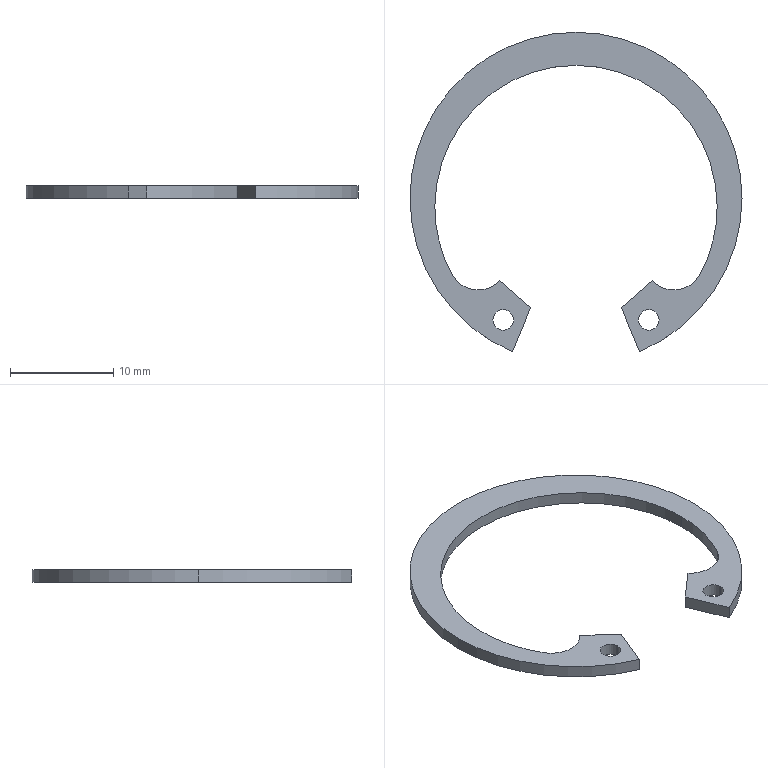Part | SolidWorks | features Extrusion 1 | 1 solid | 18 faces | box 32.1 x 30.878 x 1.2 mm | volume 280.157 mm3 | cylinder 12 | plane 6 | commonest cylinder face diameters 2 x4 27.3 x3 32.1 x3 5.6 x2
STEP:
#1=CARTESIAN_POINT('',(6.034,-11.756,0.6));
#2=VERTEX_POINT('',#1);
#3=CARTESIAN_POINT('',(8.034,-11.756,0.6));
#4=VERTEX_POINT('',#3);
#5=CARTESIAN_POINT('',(7.034,-11.756,0.6));
#6=DIRECTION('',(0.,0.,1.));
#7=DIRECTION('',(-1.,0.,0.));
#8=AXIS2_PLACEMENT_3D('',#5,#6,#7);
#9=CIRCLE('',#8,1.);
#10=EDGE_CURVE('',#2,#4,#9,.T.);
#11=ORIENTED_EDGE('',*,*,#10,.T.);
#12=CARTESIAN_POINT('',(8.034,-11.756,-0.6));
#13=VERTEX_POINT('',#12);
#14=CARTESIAN_POINT('',(8.034,-11.756,0.6));
#15=DIRECTION('',(0.,0.,-1.));
#16=VECTOR('',#15,1000.);
#17=LINE('',#14,#16);
#18=EDGE_CURVE('',#4,#13,#17,.T.);
#19=ORIENTED_EDGE('',*,*,#18,.T.);
#20=CARTESIAN_POINT('',(6.034,-11.756,-0.6));
#21=VERTEX_POINT('',#20);
#22=CARTESIAN_POINT('',(7.034,-11.756,-0.6));
#23=DIRECTION('',(0.,0.,1.));
#24=DIRECTION('',(-1.,0.,0.));
#25=AXIS2_PLACEMENT_3D('',#22,#23,#24);
#26=CIRCLE('',#25,1.);
#27=EDGE_CURVE('',#21,#13,#26,.T.);
#28=ORIENTED_EDGE('',*,*,#27,.F.);
#29=CARTESIAN_POINT('',(6.034,-11.756,0.6));
#30=DIRECTION('',(0.,0.,-1.));
#31=VECTOR('',#30,1000.);
#32=LINE('',#29,#31);
#33=EDGE_CURVE('',#2,#21,#32,.T.);
#34=ORIENTED_EDGE('',*,*,#33,.F.);
#35=EDGE_LOOP('',(#11,#19,#28,#34));
#36=FACE_OUTER_BOUND('',#35,.T.);
#37=CARTESIAN_POINT('',(7.034,-11.756,0.6));
#38=DIRECTION('',(0.,0.,-1.));
#39=DIRECTION('',(-1.,0.,0.));
#40=AXIS2_PLACEMENT_3D('',#37,#38,#39);
#41=CYLINDRICAL_SURFACE('',#40,1.);
#42=ADVANCED_FACE('',(#36),#41,.F.);
#43=CARTESIAN_POINT('',(-8.034,-11.756,0.6));
#44=VERTEX_POINT('',#43);
#45=CARTESIAN_POINT('',(-6.034,-11.756,0.6));
#46=VERTEX_POINT('',#45);
#47=CARTESIAN_POINT('',(-7.034,-11.756,0.6));
#48=DIRECTION('',(0.,0.,1.));
#49=DIRECTION('',(1.,0.,0.));
#50=AXIS2_PLACEMENT_3D('',#47,#48,#49);
#51=CIRCLE('',#50,1.);
#52=EDGE_CURVE('',#44,#46,#51,.T.);
#53=ORIENTED_EDGE('',*,*,#52,.T.);
#54=CARTESIAN_POINT('',(-6.034,-11.756,-0.6));
#55=VERTEX_POINT('',#54);
#56=CARTESIAN_POINT('',(-6.034,-11.756,0.6));
#57=DIRECTION('',(0.,0.,-1.));
#58=VECTOR('',#57,1000.);
#59=LINE('',#56,#58);
#60=EDGE_CURVE('',#46,#55,#59,.T.);
#61=ORIENTED_EDGE('',*,*,#60,.T.);
#62=CARTESIAN_POINT('',(-8.034,-11.756,-0.6));
#63=VERTEX_POINT('',#62);
#64=CARTESIAN_POINT('',(-7.034,-11.756,-0.6));
#65=DIRECTION('',(0.,0.,1.));
#66=DIRECTION('',(1.,0.,0.));
#67=AXIS2_PLACEMENT_3D('',#64,#65,#66);
#68=CIRCLE('',#67,1.);
#69=EDGE_CURVE('',#63,#55,#68,.T.);
#70=ORIENTED_EDGE('',*,*,#69,.F.);
#71=CARTESIAN_POINT('',(-8.034,-11.756,0.6));
#72=DIRECTION('',(0.,0.,-1.));
#73=VECTOR('',#72,1000.);
#74=LINE('',#71,#73);
#75=EDGE_CURVE('',#44,#63,#74,.T.);
#76=ORIENTED_EDGE('',*,*,#75,.F.);
#77=EDGE_LOOP('',(#53,#61,#70,#76));
#78=FACE_OUTER_BOUND('',#77,.T.);
#79=CARTESIAN_POINT('',(-7.034,-11.756,0.6));
#80=DIRECTION('',(0.,0.,-1.));
#81=DIRECTION('',(-1.,0.,0.));
#82=AXIS2_PLACEMENT_3D('',#79,#80,#81);
#83=CYLINDRICAL_SURFACE('',#82,1.);
#84=ADVANCED_FACE('',(#78),#83,.F.);
#85=CARTESIAN_POINT('',(13.65,-0.8,0.6));
#86=VERTEX_POINT('',#85);
#87=CARTESIAN_POINT('',(11.926,-7.44,0.6));
#88=VERTEX_POINT('',#87);
#89=CARTESIAN_POINT('',(0.,-0.8,0.6));
#90=DIRECTION('',(0.,0.,-1.));
#91=DIRECTION('',(1.,0.,0.));
#92=AXIS2_PLACEMENT_3D('',#89,#90,#91);
#93=CIRCLE('',#92,13.65);
#94=EDGE_CURVE('',#86,#88,#93,.T.);
#95=ORIENTED_EDGE('',*,*,#94,.F.);
#96=CARTESIAN_POINT('',(13.65,-0.8,-0.6));
#97=VERTEX_POINT('',#96);
#98=CARTESIAN_POINT('',(13.65,-0.8,0.6));
#99=DIRECTION('',(0.,0.,-1.));
#100=VECTOR('',#99,1000.);
#101=LINE('',#98,#100);
#102=EDGE_CURVE('',#86,#97,#101,.T.);
#103=ORIENTED_EDGE('',*,*,#102,.T.);
#104=CARTESIAN_POINT('',(11.926,-7.44,-0.6));
#105=VERTEX_POINT('',#104);
#106=CARTESIAN_POINT('',(0.,-0.8,-0.6));
#107=DIRECTION('',(0.,0.,-1.));
#108=DIRECTION('',(1.,0.,0.));
#109=AXIS2_PLACEMENT_3D('',#106,#107,#108);
#110=CIRCLE('',#109,13.65);
#111=EDGE_CURVE('',#97,#105,#110,.T.);
#112=ORIENTED_EDGE('',*,*,#111,.T.);
#113=CARTESIAN_POINT('',(11.926,-7.44,0.6));
#114=DIRECTION('',(0.,0.,-1.));
#115=VECTOR('',#114,1000.);
#116=LINE('',#113,#115);
#117=EDGE_CURVE('',#88,#105,#116,.T.);
#118=ORIENTED_EDGE('',*,*,#117,.F.);
#119=EDGE_LOOP('',(#95,#103,#112,#118));
#120=FACE_OUTER_BOUND('',#119,.T.);
#121=CARTESIAN_POINT('',(0.,-0.8,0.6));
#122=DIRECTION('',(0.,0.,-1.));
#123=DIRECTION('',(-1.,0.,0.));
#124=AXIS2_PLACEMENT_3D('',#121,#122,#123);
#125=CYLINDRICAL_SURFACE('',#124,13.65);
#126=ADVANCED_FACE('',(#120),#125,.F.);
#127=ORIENTED_EDGE('',*,*,#102,.F.);
#128=CARTESIAN_POINT('',(-13.65,-0.8,0.6));
#129=VERTEX_POINT('',#128);
#130=CARTESIAN_POINT('',(0.,-0.8,0.6));
#131=DIRECTION('',(0.,0.,-1.));
#132=DIRECTION('',(1.,0.,0.));
#133=AXIS2_PLACEMENT_3D('',#130,#131,#132);
#134=CIRCLE('',#133,13.65);
#135=EDGE_CURVE('',#129,#86,#134,.T.);
#136=ORIENTED_EDGE('',*,*,#135,.F.);
#137=CARTESIAN_POINT('',(-13.65,-0.8,-0.6));
#138=VERTEX_POINT('',#137);
#139=CARTESIAN_POINT('',(-13.65,-0.8,0.6));
#140=DIRECTION('',(0.,0.,-1.));
#141=VECTOR('',#140,1000.);
#142=LINE('',#139,#141);
#143=EDGE_CURVE('',#129,#138,#142,.T.);
#144=ORIENTED_EDGE('',*,*,#143,.T.);
#145=CARTESIAN_POINT('',(0.,-0.8,-0.6));
#146=DIRECTION('',(0.,0.,-1.));
#147=DIRECTION('',(1.,0.,0.));
#148=AXIS2_PLACEMENT_3D('',#145,#146,#147);
#149=CIRCLE('',#148,13.65);
#150=EDGE_CURVE('',#138,#97,#149,.T.);
#151=ORIENTED_EDGE('',*,*,#150,.T.);
#152=EDGE_LOOP('',(#127,#136,#144,#151));
#153=FACE_OUTER_BOUND('',#152,.T.);
#154=CARTESIAN_POINT('',(0.,-0.8,0.6));
#155=DIRECTION('',(0.,0.,-1.));
#156=DIRECTION('',(-1.,0.,0.));
#157=AXIS2_PLACEMENT_3D('',#154,#155,#156);
#158=CYLINDRICAL_SURFACE('',#157,13.65);
#159=ADVANCED_FACE('',(#153),#158,.F.);
#160=CARTESIAN_POINT('',(16.05,0.,0.6));
#161=VERTEX_POINT('',#160);
#162=CARTESIAN_POINT('',(-16.05,0.,0.6));
#163=VERTEX_POINT('',#162);
#164=CARTESIAN_POINT('',(0.,0.,0.6));
#165=DIRECTION('',(0.,0.,1.));
#166=DIRECTION('',(1.,0.,0.));
#167=AXIS2_PLACEMENT_3D('',#164,#165,#166);
#168=CIRCLE('',#167,16.05);
#169=EDGE_CURVE('',#161,#163,#168,.T.);
#170=ORIENTED_EDGE('',*,*,#169,.F.);
#171=CARTESIAN_POINT('',(16.05,0.,-0.6));
#172=VERTEX_POINT('',#171);
#173=CARTESIAN_POINT('',(16.05,0.,0.6));
#174=DIRECTION('',(0.,0.,-1.));
#175=VECTOR('',#174,1000.);
#176=LINE('',#173,#175);
#177=EDGE_CURVE('',#161,#172,#176,.T.);
#178=ORIENTED_EDGE('',*,*,#177,.T.);
#179=CARTESIAN_POINT('',(-16.05,0.,-0.6));
#180=VERTEX_POINT('',#179);
#181=CARTESIAN_POINT('',(0.,0.,-0.6));
#182=DIRECTION('',(0.,0.,1.));
#183=DIRECTION('',(1.,0.,0.));
#184=AXIS2_PLACEMENT_3D('',#181,#182,#183);
#185=CIRCLE('',#184,16.05);
#186=EDGE_CURVE('',#172,#180,#185,.T.);
#187=ORIENTED_EDGE('',*,*,#186,.T.);
#188=CARTESIAN_POINT('',(-16.05,0.,0.6));
#189=DIRECTION('',(0.,0.,-1.));
#190=VECTOR('',#189,1000.);
#191=LINE('',#188,#190);
#192=EDGE_CURVE('',#163,#180,#191,.T.);
#193=ORIENTED_EDGE('',*,*,#192,.F.);
#194=EDGE_LOOP('',(#170,#178,#187,#193));
#195=FACE_OUTER_BOUND('',#194,.T.);
#196=CARTESIAN_POINT('',(0.,0.,0.6));
#197=DIRECTION('',(0.,0.,-1.));
#198=DIRECTION('',(-1.,0.,0.));
#199=AXIS2_PLACEMENT_3D('',#196,#197,#198);
#200=CYLINDRICAL_SURFACE('',#199,16.05);
#201=ADVANCED_FACE('',(#195),#200,.T.);
#202=CARTESIAN_POINT('',(-6.142,-14.828,0.6));
#203=VERTEX_POINT('',#202);
#204=CARTESIAN_POINT('',(0.,0.,0.6));
#205=DIRECTION('',(0.,0.,1.));
#206=DIRECTION('',(1.,0.,0.));
#207=AXIS2_PLACEMENT_3D('',#204,#205,#206);
#208=CIRCLE('',#207,16.05);
#209=EDGE_CURVE('',#163,#203,#208,.T.);
#210=ORIENTED_EDGE('',*,*,#209,.F.);
#211=ORIENTED_EDGE('',*,*,#192,.T.);
#212=CARTESIAN_POINT('',(-6.142,-14.828,-0.6));
#213=VERTEX_POINT('',#212);
#214=CARTESIAN_POINT('',(0.,0.,-0.6));
#215=DIRECTION('',(0.,0.,1.));
#216=DIRECTION('',(1.,0.,0.));
#217=AXIS2_PLACEMENT_3D('',#214,#215,#216);
#218=CIRCLE('',#217,16.05);
#219=EDGE_CURVE('',#180,#213,#218,.T.);
#220=ORIENTED_EDGE('',*,*,#219,.T.);
#221=CARTESIAN_POINT('',(-6.142,-14.828,0.6));
#222=DIRECTION('',(0.,0.,-1.));
#223=VECTOR('',#222,1000.);
#224=LINE('',#221,#223);
#225=EDGE_CURVE('',#203,#213,#224,.T.);
#226=ORIENTED_EDGE('',*,*,#225,.F.);
#227=EDGE_LOOP('',(#210,#211,#220,#226));
#228=FACE_OUTER_BOUND('',#227,.T.);
#229=CARTESIAN_POINT('',(0.,0.,0.6));
#230=DIRECTION('',(0.,0.,-1.));
#231=DIRECTION('',(-1.,0.,0.));
#232=AXIS2_PLACEMENT_3D('',#229,#230,#231);
#233=CYLINDRICAL_SURFACE('',#232,16.05);
#234=ADVANCED_FACE('',(#228),#233,.T.);
#235=ORIENTED_EDGE('',*,*,#52,.F.);
#236=CARTESIAN_POINT('',(-7.034,-11.756,0.6));
#237=DIRECTION('',(0.,0.,1.));
#238=DIRECTION('',(1.,0.,0.));
#239=AXIS2_PLACEMENT_3D('',#236,#237,#238);
#240=CIRCLE('',#239,1.);
#241=EDGE_CURVE('',#46,#44,#240,.T.);
#242=ORIENTED_EDGE('',*,*,#241,.F.);
#243=EDGE_LOOP('',(#235,#242));
#244=FACE_BOUND('',#243,.T.);
#245=CARTESIAN_POINT('',(6.142,-14.828,0.6));
#246=VERTEX_POINT('',#245);
#247=CARTESIAN_POINT('',(0.,0.,0.6));
#248=DIRECTION('',(0.,0.,1.));
#249=DIRECTION('',(1.,0.,0.));
#250=AXIS2_PLACEMENT_3D('',#247,#248,#249);
#251=CIRCLE('',#250,16.05);
#252=EDGE_CURVE('',#246,#161,#251,.T.);
#253=ORIENTED_EDGE('',*,*,#252,.T.);
#254=ORIENTED_EDGE('',*,*,#169,.T.);
#255=ORIENTED_EDGE('',*,*,#209,.T.);
#256=CARTESIAN_POINT('',(-4.382,-10.578,0.6));
#257=VERTEX_POINT('',#256);
#258=CARTESIAN_POINT('',(-4.382,-10.578,0.6));
#259=DIRECTION('',(0.3827,0.9239,0.));
#260=VECTOR('',#259,1000.);
#261=LINE('',#258,#260);
#262=EDGE_CURVE('',#203,#257,#261,.T.);
#263=ORIENTED_EDGE('',*,*,#262,.T.);
#264=CARTESIAN_POINT('',(-7.38,-7.931,0.6));
#265=VERTEX_POINT('',#264);
#266=CARTESIAN_POINT('',(-7.38,-7.931,0.6));
#267=DIRECTION('',(-0.7497,0.6618,0.));
#268=VECTOR('',#267,1000.);
#269=LINE('',#266,#268);
#270=EDGE_CURVE('',#257,#265,#269,.T.);
#271=ORIENTED_EDGE('',*,*,#270,.T.);
#272=CARTESIAN_POINT('',(-11.926,-7.44,0.6));
#273=VERTEX_POINT('',#272);
#274=CARTESIAN_POINT('',(-9.48,-6.078,0.6));
#275=DIRECTION('',(0.,0.,-1.));
#276=DIRECTION('',(1.,0.,0.));
#277=AXIS2_PLACEMENT_3D('',#274,#275,#276);
#278=CIRCLE('',#277,2.8);
#279=EDGE_CURVE('',#265,#273,#278,.T.);
#280=ORIENTED_EDGE('',*,*,#279,.T.);
#281=CARTESIAN_POINT('',(0.,-0.8,0.6));
#282=DIRECTION('',(0.,0.,-1.));
#283=DIRECTION('',(1.,0.,0.));
#284=AXIS2_PLACEMENT_3D('',#281,#282,#283);
#285=CIRCLE('',#284,13.65);
#286=EDGE_CURVE('',#273,#129,#285,.T.);
#287=ORIENTED_EDGE('',*,*,#286,.T.);
#288=ORIENTED_EDGE('',*,*,#135,.T.);
#289=ORIENTED_EDGE('',*,*,#94,.T.);
#290=CARTESIAN_POINT('',(7.38,-7.931,0.6));
#291=VERTEX_POINT('',#290);
#292=CARTESIAN_POINT('',(9.48,-6.078,0.6));
#293=DIRECTION('',(0.,0.,-1.));
#294=DIRECTION('',(-1.,0.,0.));
#295=AXIS2_PLACEMENT_3D('',#292,#293,#294);
#296=CIRCLE('',#295,2.8);
#297=EDGE_CURVE('',#88,#291,#296,.T.);
#298=ORIENTED_EDGE('',*,*,#297,.T.);
#299=CARTESIAN_POINT('',(4.382,-10.578,0.6));
#300=VERTEX_POINT('',#299);
#301=CARTESIAN_POINT('',(7.38,-7.931,0.6));
#302=DIRECTION('',(-0.7497,-0.6618,0.));
#303=VECTOR('',#302,1000.);
#304=LINE('',#301,#303);
#305=EDGE_CURVE('',#291,#300,#304,.T.);
#306=ORIENTED_EDGE('',*,*,#305,.T.);
#307=CARTESIAN_POINT('',(4.382,-10.578,0.6));
#308=DIRECTION('',(0.3827,-0.9239,0.));
#309=VECTOR('',#308,1000.);
#310=LINE('',#307,#309);
#311=EDGE_CURVE('',#300,#246,#310,.T.);
#312=ORIENTED_EDGE('',*,*,#311,.T.);
#313=EDGE_LOOP('',(#253,#254,#255,#263,#271,#280,#287,#288,#289,#298,#306,#312));
#314=FACE_OUTER_BOUND('',#313,.T.);
#315=ORIENTED_EDGE('',*,*,#10,.F.);
#316=CARTESIAN_POINT('',(7.034,-11.756,0.6));
#317=DIRECTION('',(0.,0.,1.));
#318=DIRECTION('',(-1.,0.,0.));
#319=AXIS2_PLACEMENT_3D('',#316,#317,#318);
#320=CIRCLE('',#319,1.);
#321=EDGE_CURVE('',#4,#2,#320,.T.);
#322=ORIENTED_EDGE('',*,*,#321,.F.);
#323=EDGE_LOOP('',(#315,#322));
#324=FACE_BOUND('',#323,.T.);
#325=CARTESIAN_POINT('',(0.,0.,0.6));
#326=DIRECTION('',(0.,0.,1.));
#327=DIRECTION('',(1.,0.,0.));
#328=AXIS2_PLACEMENT_3D('',#325,#326,#327);
#329=PLANE('',#328);
#330=ADVANCED_FACE('',(#244,#314,#324),#329,.T.);
#331=ORIENTED_EDGE('',*,*,#177,.F.);
#332=ORIENTED_EDGE('',*,*,#252,.F.);
#333=CARTESIAN_POINT('',(6.142,-14.828,-0.6));
#334=VERTEX_POINT('',#333);
#335=CARTESIAN_POINT('',(6.142,-14.828,0.6));
#336=DIRECTION('',(0.,0.,-1.));
#337=VECTOR('',#336,1000.);
#338=LINE('',#335,#337);
#339=EDGE_CURVE('',#246,#334,#338,.T.);
#340=ORIENTED_EDGE('',*,*,#339,.T.);
#341=CARTESIAN_POINT('',(0.,0.,-0.6));
#342=DIRECTION('',(0.,0.,1.));
#343=DIRECTION('',(1.,0.,0.));
#344=AXIS2_PLACEMENT_3D('',#341,#342,#343);
#345=CIRCLE('',#344,16.05);
#346=EDGE_CURVE('',#334,#172,#345,.T.);
#347=ORIENTED_EDGE('',*,*,#346,.T.);
#348=EDGE_LOOP('',(#331,#332,#340,#347));
#349=FACE_OUTER_BOUND('',#348,.T.);
#350=CARTESIAN_POINT('',(0.,0.,0.6));
#351=DIRECTION('',(0.,0.,-1.));
#352=DIRECTION('',(-1.,0.,0.));
#353=AXIS2_PLACEMENT_3D('',#350,#351,#352);
#354=CYLINDRICAL_SURFACE('',#353,16.05);
#355=ADVANCED_FACE('',(#349),#354,.T.);
#356=ORIENTED_EDGE('',*,*,#225,.T.);
#357=CARTESIAN_POINT('',(-4.382,-10.578,-0.6));
#358=VERTEX_POINT('',#357);
#359=CARTESIAN_POINT('',(-4.382,-10.578,-0.6));
#360=DIRECTION('',(0.3827,0.9239,0.));
#361=VECTOR('',#360,1000.);
#362=LINE('',#359,#361);
#363=EDGE_CURVE('',#213,#358,#362,.T.);
#364=ORIENTED_EDGE('',*,*,#363,.T.);
#365=CARTESIAN_POINT('',(-4.382,-10.578,0.6));
#366=DIRECTION('',(0.,0.,-1.));
#367=VECTOR('',#366,1000.);
#368=LINE('',#365,#367);
#369=EDGE_CURVE('',#257,#358,#368,.T.);
#370=ORIENTED_EDGE('',*,*,#369,.F.);
#371=ORIENTED_EDGE('',*,*,#262,.F.);
#372=EDGE_LOOP('',(#356,#364,#370,#371));
#373=FACE_OUTER_BOUND('',#372,.T.);
#374=CARTESIAN_POINT('',(-4.382,-10.578,0.6));
#375=DIRECTION('',(-0.9239,0.3827,0.));
#376=DIRECTION('',(-0.3827,-0.9239,0.));
#377=AXIS2_PLACEMENT_3D('',#374,#375,#376);
#378=PLANE('',#377);
#379=ADVANCED_FACE('',(#373),#378,.F.);
#380=ORIENTED_EDGE('',*,*,#369,.T.);
#381=CARTESIAN_POINT('',(-7.38,-7.931,-0.6));
#382=VERTEX_POINT('',#381);
#383=CARTESIAN_POINT('',(-7.38,-7.931,-0.6));
#384=DIRECTION('',(-0.7497,0.6618,0.));
#385=VECTOR('',#384,1000.);
#386=LINE('',#383,#385);
#387=EDGE_CURVE('',#358,#382,#386,.T.);
#388=ORIENTED_EDGE('',*,*,#387,.T.);
#389=CARTESIAN_POINT('',(-7.38,-7.931,0.6));
#390=DIRECTION('',(0.,0.,-1.));
#391=VECTOR('',#390,1000.);
#392=LINE('',#389,#391);
#393=EDGE_CURVE('',#265,#382,#392,.T.);
#394=ORIENTED_EDGE('',*,*,#393,.F.);
#395=ORIENTED_EDGE('',*,*,#270,.F.);
#396=EDGE_LOOP('',(#380,#388,#394,#395));
#397=FACE_OUTER_BOUND('',#396,.T.);
#398=CARTESIAN_POINT('',(-7.38,-7.931,0.6));
#399=DIRECTION('',(-0.6618,-0.7497,0.));
#400=DIRECTION('',(0.7497,-0.6618,0.));
#401=AXIS2_PLACEMENT_3D('',#398,#399,#400);
#402=PLANE('',#401);
#403=ADVANCED_FACE('',(#397),#402,.F.);
#404=ORIENTED_EDGE('',*,*,#393,.T.);
#405=CARTESIAN_POINT('',(-11.926,-7.44,-0.6));
#406=VERTEX_POINT('',#405);
#407=CARTESIAN_POINT('',(-9.48,-6.078,-0.6));
#408=DIRECTION('',(0.,0.,-1.));
#409=DIRECTION('',(1.,0.,0.));
#410=AXIS2_PLACEMENT_3D('',#407,#408,#409);
#411=CIRCLE('',#410,2.8);
#412=EDGE_CURVE('',#382,#406,#411,.T.);
#413=ORIENTED_EDGE('',*,*,#412,.T.);
#414=CARTESIAN_POINT('',(-11.926,-7.44,0.6));
#415=DIRECTION('',(0.,0.,-1.));
#416=VECTOR('',#415,1000.);
#417=LINE('',#414,#416);
#418=EDGE_CURVE('',#273,#406,#417,.T.);
#419=ORIENTED_EDGE('',*,*,#418,.F.);
#420=ORIENTED_EDGE('',*,*,#279,.F.);
#421=EDGE_LOOP('',(#404,#413,#419,#420));
#422=FACE_OUTER_BOUND('',#421,.T.);
#423=CARTESIAN_POINT('',(-9.48,-6.078,0.6));
#424=DIRECTION('',(0.,0.,-1.));
#425=DIRECTION('',(-1.,0.,0.));
#426=AXIS2_PLACEMENT_3D('',#423,#424,#425);
#427=CYLINDRICAL_SURFACE('',#426,2.8);
#428=ADVANCED_FACE('',(#422),#427,.F.);
#429=ORIENTED_EDGE('',*,*,#143,.F.);
#430=ORIENTED_EDGE('',*,*,#286,.F.);
#431=ORIENTED_EDGE('',*,*,#418,.T.);
#432=CARTESIAN_POINT('',(0.,-0.8,-0.6));
#433=DIRECTION('',(0.,0.,-1.));
#434=DIRECTION('',(1.,0.,0.));
#435=AXIS2_PLACEMENT_3D('',#432,#433,#434);
#436=CIRCLE('',#435,13.65);
#437=EDGE_CURVE('',#406,#138,#436,.T.);
#438=ORIENTED_EDGE('',*,*,#437,.T.);
#439=EDGE_LOOP('',(#429,#430,#431,#438));
#440=FACE_OUTER_BOUND('',#439,.T.);
#441=CARTESIAN_POINT('',(0.,-0.8,0.6));
#442=DIRECTION('',(0.,0.,-1.));
#443=DIRECTION('',(-1.,0.,0.));
#444=AXIS2_PLACEMENT_3D('',#441,#442,#443);
#445=CYLINDRICAL_SURFACE('',#444,13.65);
#446=ADVANCED_FACE('',(#440),#445,.F.);
#447=ORIENTED_EDGE('',*,*,#117,.T.);
#448=CARTESIAN_POINT('',(7.38,-7.931,-0.6));
#449=VERTEX_POINT('',#448);
#450=CARTESIAN_POINT('',(9.48,-6.078,-0.6));
#451=DIRECTION('',(0.,0.,-1.));
#452=DIRECTION('',(-1.,0.,0.));
#453=AXIS2_PLACEMENT_3D('',#450,#451,#452);
#454=CIRCLE('',#453,2.8);
#455=EDGE_CURVE('',#105,#449,#454,.T.);
#456=ORIENTED_EDGE('',*,*,#455,.T.);
#457=CARTESIAN_POINT('',(7.38,-7.931,0.6));
#458=DIRECTION('',(0.,0.,-1.));
#459=VECTOR('',#458,1000.);
#460=LINE('',#457,#459);
#461=EDGE_CURVE('',#291,#449,#460,.T.);
#462=ORIENTED_EDGE('',*,*,#461,.F.);
#463=ORIENTED_EDGE('',*,*,#297,.F.);
#464=EDGE_LOOP('',(#447,#456,#462,#463));
#465=FACE_OUTER_BOUND('',#464,.T.);
#466=CARTESIAN_POINT('',(9.48,-6.078,0.6));
#467=DIRECTION('',(0.,0.,-1.));
#468=DIRECTION('',(-1.,0.,0.));
#469=AXIS2_PLACEMENT_3D('',#466,#467,#468);
#470=CYLINDRICAL_SURFACE('',#469,2.8);
#471=ADVANCED_FACE('',(#465),#470,.F.);
#472=ORIENTED_EDGE('',*,*,#461,.T.);
#473=CARTESIAN_POINT('',(4.382,-10.578,-0.6));
#474=VERTEX_POINT('',#473);
#475=CARTESIAN_POINT('',(7.38,-7.931,-0.6));
#476=DIRECTION('',(-0.7497,-0.6618,0.));
#477=VECTOR('',#476,1000.);
#478=LINE('',#475,#477);
#479=EDGE_CURVE('',#449,#474,#478,.T.);
#480=ORIENTED_EDGE('',*,*,#479,.T.);
#481=CARTESIAN_POINT('',(4.382,-10.578,0.6));
#482=DIRECTION('',(0.,0.,-1.));
#483=VECTOR('',#482,1000.);
#484=LINE('',#481,#483);
#485=EDGE_CURVE('',#300,#474,#484,.T.);
#486=ORIENTED_EDGE('',*,*,#485,.F.);
#487=ORIENTED_EDGE('',*,*,#305,.F.);
#488=EDGE_LOOP('',(#472,#480,#486,#487));
#489=FACE_OUTER_BOUND('',#488,.T.);
#490=CARTESIAN_POINT('',(7.38,-7.931,0.6));
#491=DIRECTION('',(0.6618,-0.7497,0.));
#492=DIRECTION('',(0.7497,0.6618,0.));
#493=AXIS2_PLACEMENT_3D('',#490,#491,#492);
#494=PLANE('',#493);
#495=ADVANCED_FACE('',(#489),#494,.F.);
#496=ORIENTED_EDGE('',*,*,#485,.T.);
#497=CARTESIAN_POINT('',(4.382,-10.578,-0.6));
#498=DIRECTION('',(0.3827,-0.9239,0.));
#499=VECTOR('',#498,1000.);
#500=LINE('',#497,#499);
#501=EDGE_CURVE('',#474,#334,#500,.T.);
#502=ORIENTED_EDGE('',*,*,#501,.T.);
#503=ORIENTED_EDGE('',*,*,#339,.F.);
#504=ORIENTED_EDGE('',*,*,#311,.F.);
#505=EDGE_LOOP('',(#496,#502,#503,#504));
#506=FACE_OUTER_BOUND('',#505,.T.);
#507=CARTESIAN_POINT('',(4.382,-10.578,0.6));
#508=DIRECTION('',(0.9239,0.3827,0.));
#509=DIRECTION('',(-0.3827,0.9239,0.));
#510=AXIS2_PLACEMENT_3D('',#507,#508,#509);
#511=PLANE('',#510);
#512=ADVANCED_FACE('',(#506),#511,.F.);
#513=ORIENTED_EDGE('',*,*,#60,.F.);
#514=ORIENTED_EDGE('',*,*,#241,.T.);
#515=ORIENTED_EDGE('',*,*,#75,.T.);
#516=CARTESIAN_POINT('',(-7.034,-11.756,-0.6));
#517=DIRECTION('',(0.,0.,1.));
#518=DIRECTION('',(1.,0.,0.));
#519=AXIS2_PLACEMENT_3D('',#516,#517,#518);
#520=CIRCLE('',#519,1.);
#521=EDGE_CURVE('',#55,#63,#520,.T.);
#522=ORIENTED_EDGE('',*,*,#521,.F.);
#523=EDGE_LOOP('',(#513,#514,#515,#522));
#524=FACE_OUTER_BOUND('',#523,.T.);
#525=CARTESIAN_POINT('',(-7.034,-11.756,0.6));
#526=DIRECTION('',(0.,0.,-1.));
#527=DIRECTION('',(-1.,0.,0.));
#528=AXIS2_PLACEMENT_3D('',#525,#526,#527);
#529=CYLINDRICAL_SURFACE('',#528,1.);
#530=ADVANCED_FACE('',(#524),#529,.F.);
#531=ORIENTED_EDGE('',*,*,#18,.F.);
#532=ORIENTED_EDGE('',*,*,#321,.T.);
#533=ORIENTED_EDGE('',*,*,#33,.T.);
#534=CARTESIAN_POINT('',(7.034,-11.756,-0.6));
#535=DIRECTION('',(0.,0.,1.));
#536=DIRECTION('',(-1.,0.,0.));
#537=AXIS2_PLACEMENT_3D('',#534,#535,#536);
#538=CIRCLE('',#537,1.);
#539=EDGE_CURVE('',#13,#21,#538,.T.);
#540=ORIENTED_EDGE('',*,*,#539,.F.);
#541=EDGE_LOOP('',(#531,#532,#533,#540));
#542=FACE_OUTER_BOUND('',#541,.T.);
#543=CARTESIAN_POINT('',(7.034,-11.756,0.6));
#544=DIRECTION('',(0.,0.,-1.));
#545=DIRECTION('',(-1.,0.,0.));
#546=AXIS2_PLACEMENT_3D('',#543,#544,#545);
#547=CYLINDRICAL_SURFACE('',#546,1.);
#548=ADVANCED_FACE('',(#542),#547,.F.);
#549=ORIENTED_EDGE('',*,*,#27,.T.);
#550=ORIENTED_EDGE('',*,*,#539,.T.);
#551=EDGE_LOOP('',(#549,#550));
#552=FACE_BOUND('',#551,.T.);
#553=ORIENTED_EDGE('',*,*,#69,.T.);
#554=ORIENTED_EDGE('',*,*,#521,.T.);
#555=EDGE_LOOP('',(#553,#554));
#556=FACE_BOUND('',#555,.T.);
#557=ORIENTED_EDGE('',*,*,#346,.F.);
#558=ORIENTED_EDGE('',*,*,#501,.F.);
#559=ORIENTED_EDGE('',*,*,#479,.F.);
#560=ORIENTED_EDGE('',*,*,#455,.F.);
#561=ORIENTED_EDGE('',*,*,#111,.F.);
#562=ORIENTED_EDGE('',*,*,#150,.F.);
#563=ORIENTED_EDGE('',*,*,#437,.F.);
#564=ORIENTED_EDGE('',*,*,#412,.F.);
#565=ORIENTED_EDGE('',*,*,#387,.F.);
#566=ORIENTED_EDGE('',*,*,#363,.F.);
#567=ORIENTED_EDGE('',*,*,#219,.F.);
#568=ORIENTED_EDGE('',*,*,#186,.F.);
#569=EDGE_LOOP('',(#557,#558,#559,#560,#561,#562,#563,#564,#565,#566,#567,#568));
#570=FACE_OUTER_BOUND('',#569,.T.);
#571=CARTESIAN_POINT('',(0.,0.,-0.6));
#572=DIRECTION('',(0.,0.,1.));
#573=DIRECTION('',(1.,0.,0.));
#574=AXIS2_PLACEMENT_3D('',#571,#572,#573);
#575=PLANE('',#574);
#576=ADVANCED_FACE('',(#552,#556,#570),#575,.F.);
#577=CLOSED_SHELL('',(#42,#84,#126,#159,#201,#234,#330,#355,#379,#403,#428,#446,#471,#495,#512,#530,#548,#576));
#578=MANIFOLD_SOLID_BREP('',#577);
#579=CARTESIAN_POINT('',(0.,0.,0.));
#580=DIRECTION('',(0.,0.,1.));
#581=DIRECTION('',(1.,0.,0.));
#582=AXIS2_PLACEMENT_3D('',#579,#580,#581);
#583=(LENGTH_UNIT()NAMED_UNIT(*)SI_UNIT(.MILLI.,.METRE.));
#584=UNCERTAINTY_MEASURE_WITH_UNIT(LENGTH_MEASURE(0.00001),#583,'','');
#585=(NAMED_UNIT(*)PLANE_ANGLE_UNIT()SI_UNIT($,.RADIAN.));
#586=(NAMED_UNIT(*)SI_UNIT($,.STERADIAN.)SOLID_ANGLE_UNIT());
#587=(GEOMETRIC_REPRESENTATION_CONTEXT(3)GLOBAL_UNCERTAINTY_ASSIGNED_CONTEXT((#584))GLOBAL_UNIT_ASSIGNED_CONTEXT((#583,#585,#586))REPRESENTATION_CONTEXT('',''));
#588=ADVANCED_BREP_SHAPE_REPRESENTATION('',(#578,#582),#587);